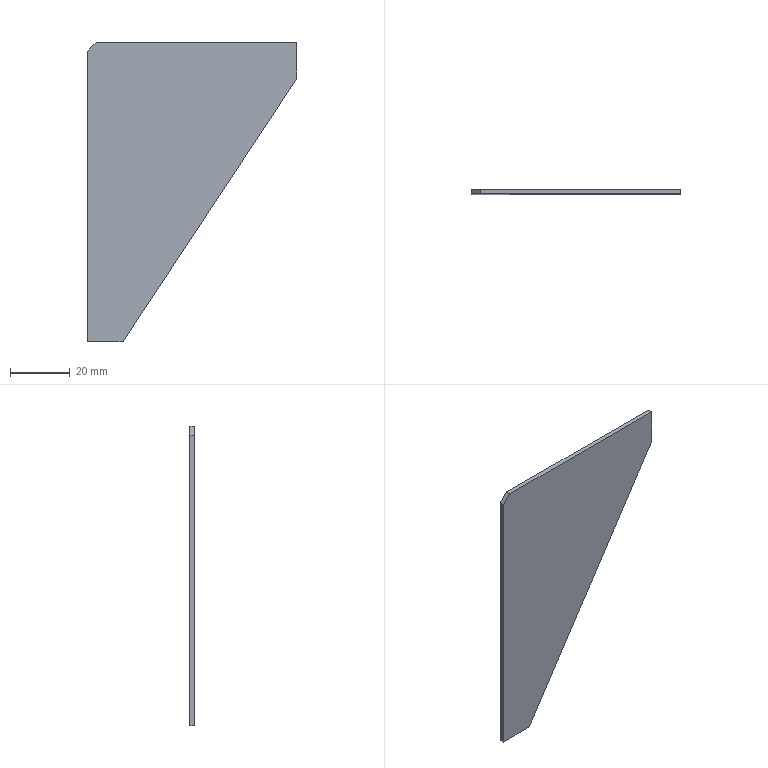Part | SolidWorks | features BaseBody 1 | 1 solid | 8 faces | box 70 x 1.5 x 100 mm | volume 6665 mm3 | plane 8
STEP:
#1=CARTESIAN_POINT('',(3.,-1.5,0.));
#2=VERTEX_POINT('',#1);
#3=CARTESIAN_POINT('',(0.,-1.5,-3.));
#4=VERTEX_POINT('',#3);
#5=CARTESIAN_POINT('',(1.5,-1.5,-1.5));
#6=DIRECTION('',(-0.7071,0.,-0.7071));
#7=VECTOR('',#6,1000.);
#8=LINE('',#5,#7);
#9=EDGE_CURVE('',#2,#4,#8,.T.);
#10=ORIENTED_EDGE('',*,*,#9,.F.);
#11=CARTESIAN_POINT('',(3.,0.,0.));
#12=VERTEX_POINT('',#11);
#13=CARTESIAN_POINT('',(3.,-1.5,0.));
#14=DIRECTION('',(0.,-1.,0.));
#15=VECTOR('',#14,1000.);
#16=LINE('',#13,#15);
#17=EDGE_CURVE('',#12,#2,#16,.T.);
#18=ORIENTED_EDGE('',*,*,#17,.F.);
#19=CARTESIAN_POINT('',(0.,0.,-3.));
#20=VERTEX_POINT('',#19);
#21=CARTESIAN_POINT('',(0.,0.,-3.));
#22=DIRECTION('',(0.7071,0.,0.7071));
#23=VECTOR('',#22,1000.);
#24=LINE('',#21,#23);
#25=EDGE_CURVE('',#20,#12,#24,.T.);
#26=ORIENTED_EDGE('',*,*,#25,.F.);
#27=CARTESIAN_POINT('',(0.,-1.5,-3.));
#28=DIRECTION('',(0.,1.,0.));
#29=VECTOR('',#28,1000.);
#30=LINE('',#27,#29);
#31=EDGE_CURVE('',#4,#20,#30,.T.);
#32=ORIENTED_EDGE('',*,*,#31,.F.);
#33=EDGE_LOOP('',(#10,#18,#26,#32));
#34=FACE_OUTER_BOUND('',#33,.T.);
#35=CARTESIAN_POINT('',(0.,-1.5,-3.));
#36=DIRECTION('',(0.7071,0.,-0.7071));
#37=DIRECTION('',(0.,-1.,0.));
#38=AXIS2_PLACEMENT_3D('',#35,#36,#37);
#39=PLANE('',#38);
#40=ADVANCED_FACE('',(#34),#39,.F.);
#41=CARTESIAN_POINT('',(0.,0.,-100.));
#42=VERTEX_POINT('',#41);
#43=CARTESIAN_POINT('',(0.,0.,0.));
#44=DIRECTION('',(0.,0.,1.));
#45=VECTOR('',#44,1000.);
#46=LINE('',#43,#45);
#47=EDGE_CURVE('',#42,#20,#46,.T.);
#48=ORIENTED_EDGE('',*,*,#47,.T.);
#49=ORIENTED_EDGE('',*,*,#25,.T.);
#50=CARTESIAN_POINT('',(70.,0.,0.));
#51=VERTEX_POINT('',#50);
#52=CARTESIAN_POINT('',(70.,0.,0.));
#53=DIRECTION('',(1.,0.,0.));
#54=VECTOR('',#53,1000.);
#55=LINE('',#52,#54);
#56=EDGE_CURVE('',#12,#51,#55,.T.);
#57=ORIENTED_EDGE('',*,*,#56,.T.);
#58=CARTESIAN_POINT('',(70.,0.,-12.));
#59=VERTEX_POINT('',#58);
#60=CARTESIAN_POINT('',(70.,0.,-12.));
#61=DIRECTION('',(0.,0.,-1.));
#62=VECTOR('',#61,1000.);
#63=LINE('',#60,#62);
#64=EDGE_CURVE('',#51,#59,#63,.T.);
#65=ORIENTED_EDGE('',*,*,#64,.T.);
#66=CARTESIAN_POINT('',(12.,0.,-100.));
#67=VERTEX_POINT('',#66);
#68=CARTESIAN_POINT('',(12.,0.,-100.));
#69=DIRECTION('',(-0.5503,0.,-0.835));
#70=VECTOR('',#69,1000.);
#71=LINE('',#68,#70);
#72=EDGE_CURVE('',#59,#67,#71,.T.);
#73=ORIENTED_EDGE('',*,*,#72,.T.);
#74=CARTESIAN_POINT('',(0.,0.,-100.));
#75=DIRECTION('',(-1.,0.,0.));
#76=VECTOR('',#75,1000.);
#77=LINE('',#74,#76);
#78=EDGE_CURVE('',#67,#42,#77,.T.);
#79=ORIENTED_EDGE('',*,*,#78,.T.);
#80=EDGE_LOOP('',(#48,#49,#57,#65,#73,#79));
#81=FACE_OUTER_BOUND('',#80,.T.);
#82=CARTESIAN_POINT('',(0.,0.,0.));
#83=DIRECTION('',(0.,-1.,0.));
#84=DIRECTION('',(0.,0.,-1.));
#85=AXIS2_PLACEMENT_3D('',#82,#83,#84);
#86=PLANE('',#85);
#87=ADVANCED_FACE('',(#81),#86,.F.);
#88=CARTESIAN_POINT('',(70.,-1.5,0.));
#89=VERTEX_POINT('',#88);
#90=CARTESIAN_POINT('',(70.,-1.5,0.));
#91=DIRECTION('',(1.,0.,0.));
#92=VECTOR('',#91,1000.);
#93=LINE('',#90,#92);
#94=EDGE_CURVE('',#2,#89,#93,.T.);
#95=ORIENTED_EDGE('',*,*,#94,.F.);
#96=ORIENTED_EDGE('',*,*,#9,.T.);
#97=CARTESIAN_POINT('',(0.,-1.5,-100.));
#98=VERTEX_POINT('',#97);
#99=CARTESIAN_POINT('',(0.,-1.5,0.));
#100=DIRECTION('',(0.,0.,1.));
#101=VECTOR('',#100,1000.);
#102=LINE('',#99,#101);
#103=EDGE_CURVE('',#98,#4,#102,.T.);
#104=ORIENTED_EDGE('',*,*,#103,.F.);
#105=CARTESIAN_POINT('',(12.,-1.5,-100.));
#106=VERTEX_POINT('',#105);
#107=CARTESIAN_POINT('',(0.,-1.5,-100.));
#108=DIRECTION('',(-1.,0.,0.));
#109=VECTOR('',#108,1000.);
#110=LINE('',#107,#109);
#111=EDGE_CURVE('',#106,#98,#110,.T.);
#112=ORIENTED_EDGE('',*,*,#111,.F.);
#113=CARTESIAN_POINT('',(70.,-1.5,-12.));
#114=VERTEX_POINT('',#113);
#115=CARTESIAN_POINT('',(12.,-1.5,-100.));
#116=DIRECTION('',(-0.5503,0.,-0.835));
#117=VECTOR('',#116,1000.);
#118=LINE('',#115,#117);
#119=EDGE_CURVE('',#114,#106,#118,.T.);
#120=ORIENTED_EDGE('',*,*,#119,.F.);
#121=CARTESIAN_POINT('',(70.,-1.5,-12.));
#122=DIRECTION('',(0.,0.,-1.));
#123=VECTOR('',#122,1000.);
#124=LINE('',#121,#123);
#125=EDGE_CURVE('',#89,#114,#124,.T.);
#126=ORIENTED_EDGE('',*,*,#125,.F.);
#127=EDGE_LOOP('',(#95,#96,#104,#112,#120,#126));
#128=FACE_OUTER_BOUND('',#127,.T.);
#129=CARTESIAN_POINT('',(0.,-1.5,0.));
#130=DIRECTION('',(0.,-1.,0.));
#131=DIRECTION('',(0.,0.,-1.));
#132=AXIS2_PLACEMENT_3D('',#129,#130,#131);
#133=PLANE('',#132);
#134=ADVANCED_FACE('',(#128),#133,.T.);
#135=ORIENTED_EDGE('',*,*,#64,.F.);
#136=CARTESIAN_POINT('',(70.,-1.5,0.));
#137=DIRECTION('',(0.,1.,0.));
#138=VECTOR('',#137,1000.);
#139=LINE('',#136,#138);
#140=EDGE_CURVE('',#89,#51,#139,.T.);
#141=ORIENTED_EDGE('',*,*,#140,.F.);
#142=ORIENTED_EDGE('',*,*,#125,.T.);
#143=CARTESIAN_POINT('',(70.,-1.5,-12.));
#144=DIRECTION('',(0.,1.,0.));
#145=VECTOR('',#144,1000.);
#146=LINE('',#143,#145);
#147=EDGE_CURVE('',#114,#59,#146,.T.);
#148=ORIENTED_EDGE('',*,*,#147,.T.);
#149=EDGE_LOOP('',(#135,#141,#142,#148));
#150=FACE_OUTER_BOUND('',#149,.T.);
#151=CARTESIAN_POINT('',(70.,-1.5,-12.));
#152=DIRECTION('',(1.,0.,0.));
#153=DIRECTION('',(0.,1.,0.));
#154=AXIS2_PLACEMENT_3D('',#151,#152,#153);
#155=PLANE('',#154);
#156=ADVANCED_FACE('',(#150),#155,.T.);
#157=ORIENTED_EDGE('',*,*,#72,.F.);
#158=ORIENTED_EDGE('',*,*,#147,.F.);
#159=ORIENTED_EDGE('',*,*,#119,.T.);
#160=CARTESIAN_POINT('',(12.,-1.5,-100.));
#161=DIRECTION('',(0.,1.,0.));
#162=VECTOR('',#161,1000.);
#163=LINE('',#160,#162);
#164=EDGE_CURVE('',#106,#67,#163,.T.);
#165=ORIENTED_EDGE('',*,*,#164,.T.);
#166=EDGE_LOOP('',(#157,#158,#159,#165));
#167=FACE_OUTER_BOUND('',#166,.T.);
#168=CARTESIAN_POINT('',(12.,-1.5,-100.));
#169=DIRECTION('',(0.835,0.,-0.5503));
#170=DIRECTION('',(0.,-1.,0.));
#171=AXIS2_PLACEMENT_3D('',#168,#169,#170);
#172=PLANE('',#171);
#173=ADVANCED_FACE('',(#167),#172,.T.);
#174=ORIENTED_EDGE('',*,*,#78,.F.);
#175=ORIENTED_EDGE('',*,*,#164,.F.);
#176=ORIENTED_EDGE('',*,*,#111,.T.);
#177=CARTESIAN_POINT('',(0.,-1.5,-100.));
#178=DIRECTION('',(0.,1.,0.));
#179=VECTOR('',#178,1000.);
#180=LINE('',#177,#179);
#181=EDGE_CURVE('',#98,#42,#180,.T.);
#182=ORIENTED_EDGE('',*,*,#181,.T.);
#183=EDGE_LOOP('',(#174,#175,#176,#182));
#184=FACE_OUTER_BOUND('',#183,.T.);
#185=CARTESIAN_POINT('',(0.,-1.5,-100.));
#186=DIRECTION('',(0.,0.,-1.));
#187=DIRECTION('',(0.,-1.,0.));
#188=AXIS2_PLACEMENT_3D('',#185,#186,#187);
#189=PLANE('',#188);
#190=ADVANCED_FACE('',(#184),#189,.T.);
#191=ORIENTED_EDGE('',*,*,#103,.T.);
#192=ORIENTED_EDGE('',*,*,#31,.T.);
#193=ORIENTED_EDGE('',*,*,#47,.F.);
#194=ORIENTED_EDGE('',*,*,#181,.F.);
#195=EDGE_LOOP('',(#191,#192,#193,#194));
#196=FACE_OUTER_BOUND('',#195,.T.);
#197=CARTESIAN_POINT('',(0.,-1.5,0.));
#198=DIRECTION('',(-1.,0.,0.));
#199=DIRECTION('',(0.,0.,1.));
#200=AXIS2_PLACEMENT_3D('',#197,#198,#199);
#201=PLANE('',#200);
#202=ADVANCED_FACE('',(#196),#201,.T.);
#203=ORIENTED_EDGE('',*,*,#56,.F.);
#204=ORIENTED_EDGE('',*,*,#17,.T.);
#205=ORIENTED_EDGE('',*,*,#94,.T.);
#206=ORIENTED_EDGE('',*,*,#140,.T.);
#207=EDGE_LOOP('',(#203,#204,#205,#206));
#208=FACE_OUTER_BOUND('',#207,.T.);
#209=CARTESIAN_POINT('',(70.,-1.5,0.));
#210=DIRECTION('',(0.,0.,1.));
#211=DIRECTION('',(1.,0.,0.));
#212=AXIS2_PLACEMENT_3D('',#209,#210,#211);
#213=PLANE('',#212);
#214=ADVANCED_FACE('',(#208),#213,.T.);
#215=CLOSED_SHELL('',(#40,#87,#134,#156,#173,#190,#202,#214));
#216=MANIFOLD_SOLID_BREP('',#215);
#217=CARTESIAN_POINT('',(0.,0.,0.));
#218=DIRECTION('',(0.,0.,1.));
#219=DIRECTION('',(1.,0.,0.));
#220=AXIS2_PLACEMENT_3D('',#217,#218,#219);
#221=(LENGTH_UNIT()NAMED_UNIT(*)SI_UNIT(.MILLI.,.METRE.));
#222=UNCERTAINTY_MEASURE_WITH_UNIT(LENGTH_MEASURE(0.00001),#221,'','');
#223=(NAMED_UNIT(*)PLANE_ANGLE_UNIT()SI_UNIT($,.RADIAN.));
#224=(NAMED_UNIT(*)SI_UNIT($,.STERADIAN.)SOLID_ANGLE_UNIT());
#225=(GEOMETRIC_REPRESENTATION_CONTEXT(3)GLOBAL_UNCERTAINTY_ASSIGNED_CONTEXT((#222))GLOBAL_UNIT_ASSIGNED_CONTEXT((#221,#223,#224))REPRESENTATION_CONTEXT('',''));
#226=ADVANCED_BREP_SHAPE_REPRESENTATION('',(#216,#220),#225);